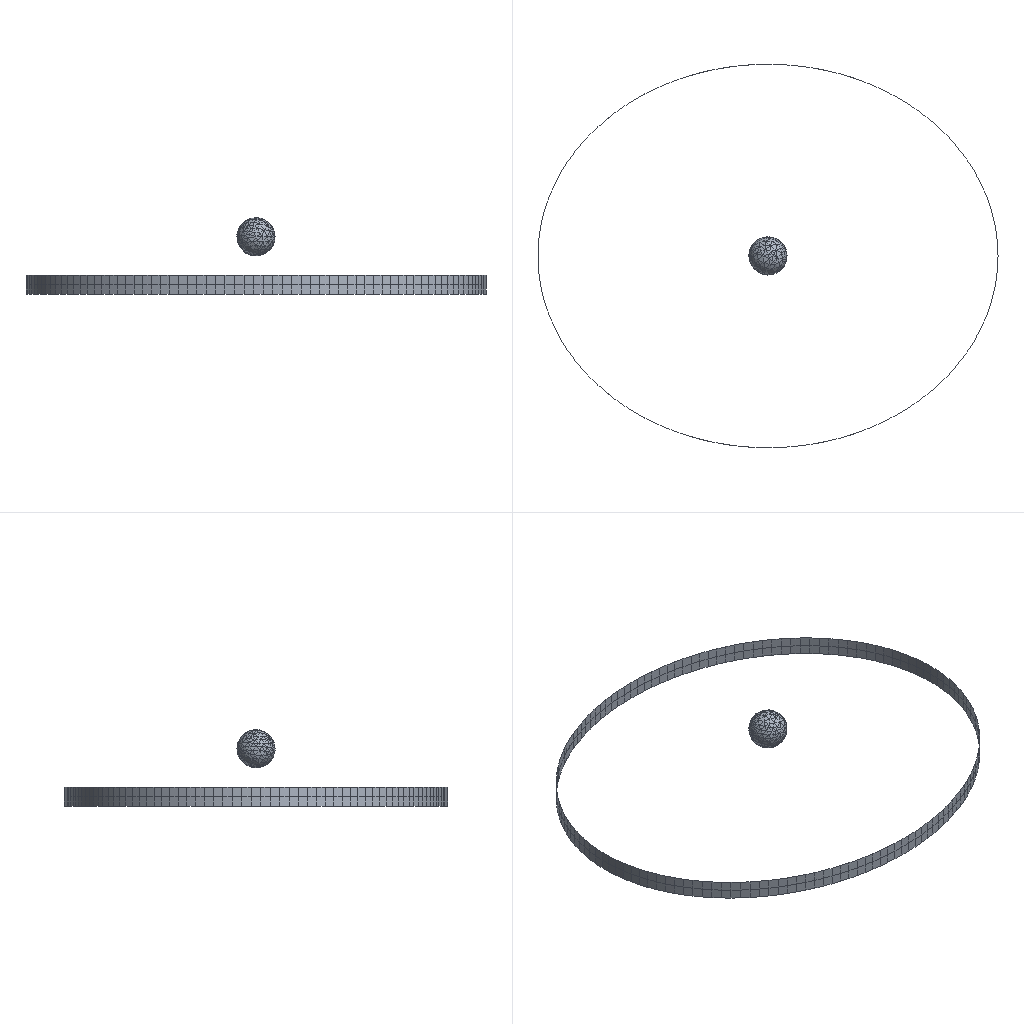Simulation study | abaqus
Set-up summary:
category,name,step,type,value,unit,region
solver,abaqus
solver,version,,,Abaqus/Explicit 2020
units,not stated in the deck,,not stated
analysis,deck,,transient,transient
load_step,Step-1,Step-1,transient
load_step,requested,,,1
mesh,nodes,,,3846
mesh,elements,,,3197
element_type,S4R,,shell,278
element_type,T3D2,,truss,1504
element_type,C3D10M,,solid,1415
load,load commands in deck,,count,1
bc,support commands in deck,,count,1
material,FRAME,,in results
material,NET,,in results
material,QIU,,in results
check,setup vs results,,match,"per instance, exact: element labels, types and connectivity; labels of the nodes the elements use; coordinates of those nodes at SINGLE_PRECISION in 3 of 3 instance(s)"
Abaqus input file, long lists of numbers shortened:
*Heading
** Job name: Job-1 Model name: Model-1
** Generated by: Abaqus/CAE 2020
*Preprint, echo=NO, model=NO, history=NO, contact=NO
**
** PARTS
**
*Part, name=Part-1
*Node
      1,   119.851,   -4.98,           0.
      2,   119.406,   -9.941,           0.
** (415 more lines like these left out)
*Element, type=S4R
  1, 139,   1, 140, 278
  2,   1,   2, 141, 140
** (276 more lines like these left out)
*Nset, nset=Set-1, generate
   1,  417,    1
*Elset, elset=Set-1, generate
   1,  278,    1
** Section: Section-1
*Shell Section, elset=Set-1, material=frame
10., 5
*End Part
**
*Part, name=net
*Node
      1,          60.,   86.603,           0.
      2,          60.,          80.,           0.
** (1171 more lines like these left out)
*Element, type=T3D2
1, 1, 2
2,   2, 450
** (1502 more lines like these left out)
*Nset, nset=Set-1, generate
    1,  1173,     1
*Elset, elset=Set-1, generate
    1,  1504,     1
** Section: net
*Solid Section, elset=Set-1, material=net
78.5,
*End Part
**
*Part, name=qiu
*Node
      1,   3.09,    9.511,           0.
      2,   5.878,   8.09,           0.
** (2254 more lines like these left out)
*Element, type=C3D10M
   1,  173,  174,  175,  176,  339,  338,  337,  341,  340,  342
   2,  173,  177,  178,  175,  345,  344,  343,  337,  346,  347
** (1413 more lines like these left out)
*Nset, nset=Set-1, generate
    1,  2256,     1
*Elset, elset=Set-1, generate
    1,  1415,     1
** Section: qiu
*Solid Section, elset=Set-1, material=qiu
,
*End Part
**
**
** ASSEMBLY
**
*Assembly, name=Assembly
**
*Instance, name=Part-1-1, part=Part-1
*End Instance
**
*Instance, name=net-1, part=net
          0.,           0.,          -5.
*End Instance
**
*Instance, name=qiu-1, part=qiu
          0.,           0.,          20.
*End Instance
**
*Nset, nset=Set-2, instance=Part-1-1, generate
   1,  417,    1
*Elset, elset=Set-2, instance=Part-1-1, generate
   1,  278,    1
*Nset, nset=Set-3, instance=net-1, generate
    1,  1173,     1
*Elset, elset=Set-3, instance=net-1, generate
    1,  1504,     1
*Nset, nset=Set-4, instance=qiu-1, generate
    1,  2256,     1
*Elset, elset=Set-4, instance=qiu-1, generate
    1,  1415,     1
*Nset, nset=s_Set-1, instance=net-1
   1,  19,  23,  27,  32,  38,  45,  53,  62,  72,  83,  95, 107, 120, 126, 154
 169, 184, 200, 202, 203, 215, 221, 245, 246, 247, 257, 258, 260, 266, 267, 283
** (3 more lines like these left out)
*Elset, elset=_m_Surf-1_SNEG, internal, instance=Part-1-1, generate
   1,  278,    1
*Surface, type=ELEMENT, name=m_Surf-1
_m_Surf-1_SNEG, SNEG
*Surface, type=NODE, name=s_Set-1_CNS_, internal
s_Set-1, 1.
** Constraint: Constraint-1
*Tie, name=Constraint-1, adjust=yes
s_Set-1_CNS_, m_Surf-1
*End Assembly
**
** MATERIALS
**
*Material, name=frame
*Density
 2e-09,
*Elastic
20000., 0.3
*Material, name=net
*Density
 1e-09,
*Elastic
50000., 0.35
*Material, name=qiu
*Density
 1.5e-09,
*Elastic
20000., 0.3
**
** INTERACTION PROPERTIES
**
*Surface Interaction, name=IntProp-1
*Friction
 0.5,
*Surface Behavior, pressure-overclosure=HARD
**
** PREDEFINED FIELDS
**
** Name: Predefined Field-1   Type: Stress
*Initial Conditions, type=STRESS
Set-3, 1.5, 1.5, 1.5,
** Name: Predefined Field-2   Type: Velocity
*Initial Conditions, type=VELOCITY
Set-4, 1, 0.
Set-4, 2, 0.
Set-4, 3, -100000.
** ----------------------------------------------------------------
**
** STEP: Step-1
**
*Step, name=Step-1, nlgeom=YES
*Dynamic, Explicit
, 0.1
*Bulk Viscosity
0.06, 1.2
**
** BOUNDARY CONDITIONS
**
** Name: BC-1 Type: 对称/反对称/完全固定
*Boundary
Set-2, ENCASTRE
**
** INTERACTIONS
**
** Interaction: Int-1
*Contact, op=NEW
*Contact Inclusions, ALL EXTERIOR
*Contact Property Assignment
 ,  , IntProp-1
**
** OUTPUT REQUESTS
**
*Restart, write, number interval=1, time marks=NO
**
** FIELD OUTPUT: F-Output-1
**
*Output, field, number interval=50
*Node Output
A, CF, RF, RM, RT, U, V
*Element Output, directions=YES
E, EVF, LE, MISES, MISESMAX, PE, PEEQ, PEEQVAVG, PEVAVG, S, SF, SVAVG
*Contact Output
CDISP, CSTRESS
**
** HISTORY OUTPUT: H-Output-1
**
*Output, history, variable=PRESELECT
*End Step
Results summary:
result,step,Step-1,partial,increments=183131 time=0.0126/0.1
result,analysis,,,transient
result,last_loadstep,,,1
result,primary field,,,"U, UR"
result,reaction total,,FX,-4595.574,model units
result,reaction total,,FY,4019.435,model units
result,reaction total,,FZ,-5765.924,model units